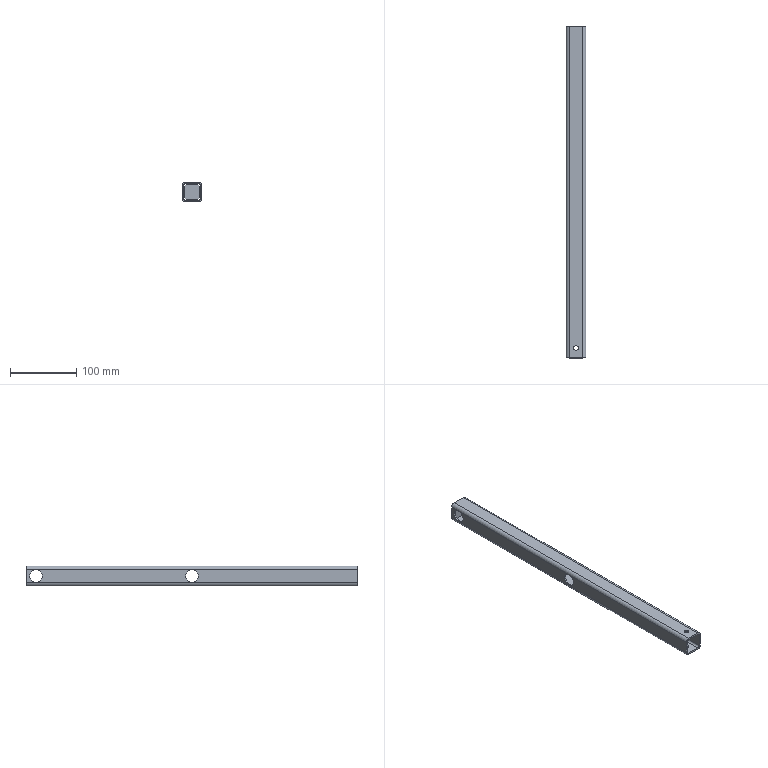Part | STEP file | 2 solids | 40 faces | box 30 x 500 x 30 mm | volume 133136 mm3 | plane 20 | cylinder 20 | commonest cylinder face diameters 19 x8 5.2 x4 7 x4 10.4 x4